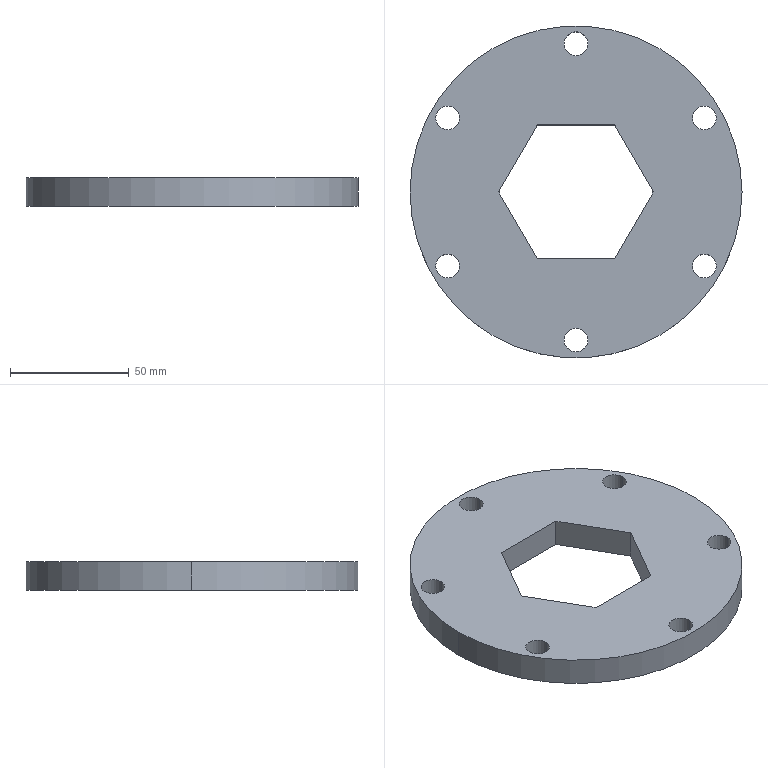Part | SolidWorks | features Extrusion 1 | 1 solid | 22 faces | box 140 x 140 x 12 mm | volume 145896 mm3 | cylinder 14 | plane 8 | commonest cylinder face diameters 10 x12 140 x2
STEP:
#1=CARTESIAN_POINT('',(-59.127,31.25,12.));
#2=VERTEX_POINT('',#1);
#3=CARTESIAN_POINT('',(-49.127,31.25,12.));
#4=VERTEX_POINT('',#3);
#5=CARTESIAN_POINT('',(-54.127,31.25,12.));
#6=DIRECTION('',(0.,0.,1.));
#7=DIRECTION('',(1.,0.,0.));
#8=AXIS2_PLACEMENT_3D('',#5,#6,#7);
#9=CIRCLE('',#8,5.);
#10=EDGE_CURVE('',#2,#4,#9,.T.);
#11=ORIENTED_EDGE('',*,*,#10,.T.);
#12=CARTESIAN_POINT('',(-49.127,31.25,0.));
#13=VERTEX_POINT('',#12);
#14=CARTESIAN_POINT('',(-49.127,31.25,12.));
#15=DIRECTION('',(0.,0.,-1.));
#16=VECTOR('',#15,1000.);
#17=LINE('',#14,#16);
#18=EDGE_CURVE('',#4,#13,#17,.T.);
#19=ORIENTED_EDGE('',*,*,#18,.T.);
#20=CARTESIAN_POINT('',(-59.127,31.25,0.));
#21=VERTEX_POINT('',#20);
#22=CARTESIAN_POINT('',(-54.127,31.25,0.));
#23=DIRECTION('',(0.,0.,1.));
#24=DIRECTION('',(1.,0.,0.));
#25=AXIS2_PLACEMENT_3D('',#22,#23,#24);
#26=CIRCLE('',#25,5.);
#27=EDGE_CURVE('',#21,#13,#26,.T.);
#28=ORIENTED_EDGE('',*,*,#27,.F.);
#29=CARTESIAN_POINT('',(-59.127,31.25,12.));
#30=DIRECTION('',(0.,0.,-1.));
#31=VECTOR('',#30,1000.);
#32=LINE('',#29,#31);
#33=EDGE_CURVE('',#2,#21,#32,.T.);
#34=ORIENTED_EDGE('',*,*,#33,.F.);
#35=EDGE_LOOP('',(#11,#19,#28,#34));
#36=FACE_OUTER_BOUND('',#35,.T.);
#37=CARTESIAN_POINT('',(-54.127,31.25,12.));
#38=DIRECTION('',(0.,0.,-1.));
#39=DIRECTION('',(-1.,0.,0.));
#40=AXIS2_PLACEMENT_3D('',#37,#38,#39);
#41=CYLINDRICAL_SURFACE('',#40,5.);
#42=ADVANCED_FACE('',(#36),#41,.F.);
#43=CARTESIAN_POINT('',(-59.127,-31.25,12.));
#44=VERTEX_POINT('',#43);
#45=CARTESIAN_POINT('',(-49.127,-31.25,12.));
#46=VERTEX_POINT('',#45);
#47=CARTESIAN_POINT('',(-54.127,-31.25,12.));
#48=DIRECTION('',(0.,0.,1.));
#49=DIRECTION('',(1.,0.,0.));
#50=AXIS2_PLACEMENT_3D('',#47,#48,#49);
#51=CIRCLE('',#50,5.);
#52=EDGE_CURVE('',#44,#46,#51,.T.);
#53=ORIENTED_EDGE('',*,*,#52,.T.);
#54=CARTESIAN_POINT('',(-49.127,-31.25,0.));
#55=VERTEX_POINT('',#54);
#56=CARTESIAN_POINT('',(-49.127,-31.25,12.));
#57=DIRECTION('',(0.,0.,-1.));
#58=VECTOR('',#57,1000.);
#59=LINE('',#56,#58);
#60=EDGE_CURVE('',#46,#55,#59,.T.);
#61=ORIENTED_EDGE('',*,*,#60,.T.);
#62=CARTESIAN_POINT('',(-59.127,-31.25,0.));
#63=VERTEX_POINT('',#62);
#64=CARTESIAN_POINT('',(-54.127,-31.25,0.));
#65=DIRECTION('',(0.,0.,1.));
#66=DIRECTION('',(1.,0.,0.));
#67=AXIS2_PLACEMENT_3D('',#64,#65,#66);
#68=CIRCLE('',#67,5.);
#69=EDGE_CURVE('',#63,#55,#68,.T.);
#70=ORIENTED_EDGE('',*,*,#69,.F.);
#71=CARTESIAN_POINT('',(-59.127,-31.25,12.));
#72=DIRECTION('',(0.,0.,-1.));
#73=VECTOR('',#72,1000.);
#74=LINE('',#71,#73);
#75=EDGE_CURVE('',#44,#63,#74,.T.);
#76=ORIENTED_EDGE('',*,*,#75,.F.);
#77=EDGE_LOOP('',(#53,#61,#70,#76));
#78=FACE_OUTER_BOUND('',#77,.T.);
#79=CARTESIAN_POINT('',(-54.127,-31.25,12.));
#80=DIRECTION('',(0.,0.,-1.));
#81=DIRECTION('',(-1.,0.,0.));
#82=AXIS2_PLACEMENT_3D('',#79,#80,#81);
#83=CYLINDRICAL_SURFACE('',#82,5.);
#84=ADVANCED_FACE('',(#78),#83,.F.);
#85=CARTESIAN_POINT('',(-5.,-62.5,12.));
#86=VERTEX_POINT('',#85);
#87=CARTESIAN_POINT('',(5.,-62.5,12.));
#88=VERTEX_POINT('',#87);
#89=CARTESIAN_POINT('',(0.,-62.5,12.));
#90=DIRECTION('',(0.,0.,1.));
#91=DIRECTION('',(1.,0.,0.));
#92=AXIS2_PLACEMENT_3D('',#89,#90,#91);
#93=CIRCLE('',#92,5.);
#94=EDGE_CURVE('',#86,#88,#93,.T.);
#95=ORIENTED_EDGE('',*,*,#94,.T.);
#96=CARTESIAN_POINT('',(5.,-62.5,0.));
#97=VERTEX_POINT('',#96);
#98=CARTESIAN_POINT('',(5.,-62.5,12.));
#99=DIRECTION('',(0.,0.,-1.));
#100=VECTOR('',#99,1000.);
#101=LINE('',#98,#100);
#102=EDGE_CURVE('',#88,#97,#101,.T.);
#103=ORIENTED_EDGE('',*,*,#102,.T.);
#104=CARTESIAN_POINT('',(-5.,-62.5,0.));
#105=VERTEX_POINT('',#104);
#106=CARTESIAN_POINT('',(0.,-62.5,0.));
#107=DIRECTION('',(0.,0.,1.));
#108=DIRECTION('',(1.,0.,0.));
#109=AXIS2_PLACEMENT_3D('',#106,#107,#108);
#110=CIRCLE('',#109,5.);
#111=EDGE_CURVE('',#105,#97,#110,.T.);
#112=ORIENTED_EDGE('',*,*,#111,.F.);
#113=CARTESIAN_POINT('',(-5.,-62.5,12.));
#114=DIRECTION('',(0.,0.,-1.));
#115=VECTOR('',#114,1000.);
#116=LINE('',#113,#115);
#117=EDGE_CURVE('',#86,#105,#116,.T.);
#118=ORIENTED_EDGE('',*,*,#117,.F.);
#119=EDGE_LOOP('',(#95,#103,#112,#118));
#120=FACE_OUTER_BOUND('',#119,.T.);
#121=CARTESIAN_POINT('',(0.,-62.5,12.));
#122=DIRECTION('',(0.,0.,-1.));
#123=DIRECTION('',(-1.,0.,0.));
#124=AXIS2_PLACEMENT_3D('',#121,#122,#123);
#125=CYLINDRICAL_SURFACE('',#124,5.);
#126=ADVANCED_FACE('',(#120),#125,.F.);
#127=CARTESIAN_POINT('',(49.127,-31.25,12.));
#128=VERTEX_POINT('',#127);
#129=CARTESIAN_POINT('',(59.127,-31.25,12.));
#130=VERTEX_POINT('',#129);
#131=CARTESIAN_POINT('',(54.127,-31.25,12.));
#132=DIRECTION('',(0.,0.,1.));
#133=DIRECTION('',(1.,0.,0.));
#134=AXIS2_PLACEMENT_3D('',#131,#132,#133);
#135=CIRCLE('',#134,5.);
#136=EDGE_CURVE('',#128,#130,#135,.T.);
#137=ORIENTED_EDGE('',*,*,#136,.T.);
#138=CARTESIAN_POINT('',(59.127,-31.25,0.));
#139=VERTEX_POINT('',#138);
#140=CARTESIAN_POINT('',(59.127,-31.25,12.));
#141=DIRECTION('',(0.,0.,-1.));
#142=VECTOR('',#141,1000.);
#143=LINE('',#140,#142);
#144=EDGE_CURVE('',#130,#139,#143,.T.);
#145=ORIENTED_EDGE('',*,*,#144,.T.);
#146=CARTESIAN_POINT('',(49.127,-31.25,0.));
#147=VERTEX_POINT('',#146);
#148=CARTESIAN_POINT('',(54.127,-31.25,0.));
#149=DIRECTION('',(0.,0.,1.));
#150=DIRECTION('',(1.,0.,0.));
#151=AXIS2_PLACEMENT_3D('',#148,#149,#150);
#152=CIRCLE('',#151,5.);
#153=EDGE_CURVE('',#147,#139,#152,.T.);
#154=ORIENTED_EDGE('',*,*,#153,.F.);
#155=CARTESIAN_POINT('',(49.127,-31.25,12.));
#156=DIRECTION('',(0.,0.,-1.));
#157=VECTOR('',#156,1000.);
#158=LINE('',#155,#157);
#159=EDGE_CURVE('',#128,#147,#158,.T.);
#160=ORIENTED_EDGE('',*,*,#159,.F.);
#161=EDGE_LOOP('',(#137,#145,#154,#160));
#162=FACE_OUTER_BOUND('',#161,.T.);
#163=CARTESIAN_POINT('',(54.127,-31.25,12.));
#164=DIRECTION('',(0.,0.,-1.));
#165=DIRECTION('',(-1.,0.,0.));
#166=AXIS2_PLACEMENT_3D('',#163,#164,#165);
#167=CYLINDRICAL_SURFACE('',#166,5.);
#168=ADVANCED_FACE('',(#162),#167,.F.);
#169=CARTESIAN_POINT('',(49.127,31.25,12.));
#170=VERTEX_POINT('',#169);
#171=CARTESIAN_POINT('',(59.127,31.25,12.));
#172=VERTEX_POINT('',#171);
#173=CARTESIAN_POINT('',(54.127,31.25,12.));
#174=DIRECTION('',(0.,0.,1.));
#175=DIRECTION('',(1.,0.,0.));
#176=AXIS2_PLACEMENT_3D('',#173,#174,#175);
#177=CIRCLE('',#176,5.);
#178=EDGE_CURVE('',#170,#172,#177,.T.);
#179=ORIENTED_EDGE('',*,*,#178,.T.);
#180=CARTESIAN_POINT('',(59.127,31.25,0.));
#181=VERTEX_POINT('',#180);
#182=CARTESIAN_POINT('',(59.127,31.25,12.));
#183=DIRECTION('',(0.,0.,-1.));
#184=VECTOR('',#183,1000.);
#185=LINE('',#182,#184);
#186=EDGE_CURVE('',#172,#181,#185,.T.);
#187=ORIENTED_EDGE('',*,*,#186,.T.);
#188=CARTESIAN_POINT('',(49.127,31.25,0.));
#189=VERTEX_POINT('',#188);
#190=CARTESIAN_POINT('',(54.127,31.25,0.));
#191=DIRECTION('',(0.,0.,1.));
#192=DIRECTION('',(1.,0.,0.));
#193=AXIS2_PLACEMENT_3D('',#190,#191,#192);
#194=CIRCLE('',#193,5.);
#195=EDGE_CURVE('',#189,#181,#194,.T.);
#196=ORIENTED_EDGE('',*,*,#195,.F.);
#197=CARTESIAN_POINT('',(49.127,31.25,12.));
#198=DIRECTION('',(0.,0.,-1.));
#199=VECTOR('',#198,1000.);
#200=LINE('',#197,#199);
#201=EDGE_CURVE('',#170,#189,#200,.T.);
#202=ORIENTED_EDGE('',*,*,#201,.F.);
#203=EDGE_LOOP('',(#179,#187,#196,#202));
#204=FACE_OUTER_BOUND('',#203,.T.);
#205=CARTESIAN_POINT('',(54.127,31.25,12.));
#206=DIRECTION('',(0.,0.,-1.));
#207=DIRECTION('',(-1.,0.,0.));
#208=AXIS2_PLACEMENT_3D('',#205,#206,#207);
#209=CYLINDRICAL_SURFACE('',#208,5.);
#210=ADVANCED_FACE('',(#204),#209,.F.);
#211=CARTESIAN_POINT('',(-5.,62.5,12.));
#212=VERTEX_POINT('',#211);
#213=CARTESIAN_POINT('',(5.,62.5,12.));
#214=VERTEX_POINT('',#213);
#215=CARTESIAN_POINT('',(0.,62.5,12.));
#216=DIRECTION('',(0.,0.,1.));
#217=DIRECTION('',(1.,0.,0.));
#218=AXIS2_PLACEMENT_3D('',#215,#216,#217);
#219=CIRCLE('',#218,5.);
#220=EDGE_CURVE('',#212,#214,#219,.T.);
#221=ORIENTED_EDGE('',*,*,#220,.T.);
#222=CARTESIAN_POINT('',(5.,62.5,0.));
#223=VERTEX_POINT('',#222);
#224=CARTESIAN_POINT('',(5.,62.5,12.));
#225=DIRECTION('',(0.,0.,-1.));
#226=VECTOR('',#225,1000.);
#227=LINE('',#224,#226);
#228=EDGE_CURVE('',#214,#223,#227,.T.);
#229=ORIENTED_EDGE('',*,*,#228,.T.);
#230=CARTESIAN_POINT('',(-5.,62.5,0.));
#231=VERTEX_POINT('',#230);
#232=CARTESIAN_POINT('',(0.,62.5,0.));
#233=DIRECTION('',(0.,0.,1.));
#234=DIRECTION('',(1.,0.,0.));
#235=AXIS2_PLACEMENT_3D('',#232,#233,#234);
#236=CIRCLE('',#235,5.);
#237=EDGE_CURVE('',#231,#223,#236,.T.);
#238=ORIENTED_EDGE('',*,*,#237,.F.);
#239=CARTESIAN_POINT('',(-5.,62.5,12.));
#240=DIRECTION('',(0.,0.,-1.));
#241=VECTOR('',#240,1000.);
#242=LINE('',#239,#241);
#243=EDGE_CURVE('',#212,#231,#242,.T.);
#244=ORIENTED_EDGE('',*,*,#243,.F.);
#245=EDGE_LOOP('',(#221,#229,#238,#244));
#246=FACE_OUTER_BOUND('',#245,.T.);
#247=CARTESIAN_POINT('',(0.,62.5,12.));
#248=DIRECTION('',(0.,0.,-1.));
#249=DIRECTION('',(-1.,0.,0.));
#250=AXIS2_PLACEMENT_3D('',#247,#248,#249);
#251=CYLINDRICAL_SURFACE('',#250,5.);
#252=ADVANCED_FACE('',(#246),#251,.F.);
#253=CARTESIAN_POINT('',(70.,0.,12.));
#254=VERTEX_POINT('',#253);
#255=CARTESIAN_POINT('',(-70.,0.,12.));
#256=VERTEX_POINT('',#255);
#257=CARTESIAN_POINT('',(0.,0.,12.));
#258=DIRECTION('',(0.,0.,1.));
#259=DIRECTION('',(1.,0.,0.));
#260=AXIS2_PLACEMENT_3D('',#257,#258,#259);
#261=CIRCLE('',#260,70.);
#262=EDGE_CURVE('',#254,#256,#261,.T.);
#263=ORIENTED_EDGE('',*,*,#262,.F.);
#264=CARTESIAN_POINT('',(70.,0.,0.));
#265=VERTEX_POINT('',#264);
#266=CARTESIAN_POINT('',(70.,0.,12.));
#267=DIRECTION('',(0.,0.,-1.));
#268=VECTOR('',#267,1000.);
#269=LINE('',#266,#268);
#270=EDGE_CURVE('',#254,#265,#269,.T.);
#271=ORIENTED_EDGE('',*,*,#270,.T.);
#272=CARTESIAN_POINT('',(-70.,0.,0.));
#273=VERTEX_POINT('',#272);
#274=CARTESIAN_POINT('',(0.,0.,0.));
#275=DIRECTION('',(0.,0.,1.));
#276=DIRECTION('',(1.,0.,0.));
#277=AXIS2_PLACEMENT_3D('',#274,#275,#276);
#278=CIRCLE('',#277,70.);
#279=EDGE_CURVE('',#265,#273,#278,.T.);
#280=ORIENTED_EDGE('',*,*,#279,.T.);
#281=CARTESIAN_POINT('',(-70.,0.,12.));
#282=DIRECTION('',(0.,0.,-1.));
#283=VECTOR('',#282,1000.);
#284=LINE('',#281,#283);
#285=EDGE_CURVE('',#256,#273,#284,.T.);
#286=ORIENTED_EDGE('',*,*,#285,.F.);
#287=EDGE_LOOP('',(#263,#271,#280,#286));
#288=FACE_OUTER_BOUND('',#287,.T.);
#289=CARTESIAN_POINT('',(0.,0.,12.));
#290=DIRECTION('',(0.,0.,-1.));
#291=DIRECTION('',(-1.,0.,0.));
#292=AXIS2_PLACEMENT_3D('',#289,#290,#291);
#293=CYLINDRICAL_SURFACE('',#292,70.);
#294=ADVANCED_FACE('',(#288),#293,.T.);
#295=ORIENTED_EDGE('',*,*,#52,.F.);
#296=CARTESIAN_POINT('',(-54.127,-31.25,12.));
#297=DIRECTION('',(0.,0.,1.));
#298=DIRECTION('',(1.,0.,0.));
#299=AXIS2_PLACEMENT_3D('',#296,#297,#298);
#300=CIRCLE('',#299,5.);
#301=EDGE_CURVE('',#46,#44,#300,.T.);
#302=ORIENTED_EDGE('',*,*,#301,.F.);
#303=EDGE_LOOP('',(#295,#302));
#304=FACE_BOUND('',#303,.T.);
#305=ORIENTED_EDGE('',*,*,#136,.F.);
#306=CARTESIAN_POINT('',(54.127,-31.25,12.));
#307=DIRECTION('',(0.,0.,1.));
#308=DIRECTION('',(1.,0.,0.));
#309=AXIS2_PLACEMENT_3D('',#306,#307,#308);
#310=CIRCLE('',#309,5.);
#311=EDGE_CURVE('',#130,#128,#310,.T.);
#312=ORIENTED_EDGE('',*,*,#311,.F.);
#313=EDGE_LOOP('',(#305,#312));
#314=FACE_BOUND('',#313,.T.);
#315=CARTESIAN_POINT('',(32.62,0.,12.));
#316=VERTEX_POINT('',#315);
#317=CARTESIAN_POINT('',(16.31,28.25,12.));
#318=VERTEX_POINT('',#317);
#319=CARTESIAN_POINT('',(32.62,0.,12.));
#320=DIRECTION('',(-0.5,0.866,0.));
#321=VECTOR('',#320,1000.);
#322=LINE('',#319,#321);
#323=EDGE_CURVE('',#316,#318,#322,.T.);
#324=ORIENTED_EDGE('',*,*,#323,.F.);
#325=CARTESIAN_POINT('',(16.31,-28.25,12.));
#326=VERTEX_POINT('',#325);
#327=CARTESIAN_POINT('',(16.31,-28.25,12.));
#328=DIRECTION('',(0.5,0.866,0.));
#329=VECTOR('',#328,1000.);
#330=LINE('',#327,#329);
#331=EDGE_CURVE('',#326,#316,#330,.T.);
#332=ORIENTED_EDGE('',*,*,#331,.F.);
#333=CARTESIAN_POINT('',(-16.31,-28.25,12.));
#334=VERTEX_POINT('',#333);
#335=CARTESIAN_POINT('',(-16.31,-28.25,12.));
#336=DIRECTION('',(1.,0.,0.));
#337=VECTOR('',#336,1000.);
#338=LINE('',#335,#337);
#339=EDGE_CURVE('',#334,#326,#338,.T.);
#340=ORIENTED_EDGE('',*,*,#339,.F.);
#341=CARTESIAN_POINT('',(-32.62,0.,12.));
#342=VERTEX_POINT('',#341);
#343=CARTESIAN_POINT('',(-32.62,0.,12.));
#344=DIRECTION('',(0.5,-0.866,0.));
#345=VECTOR('',#344,1000.);
#346=LINE('',#343,#345);
#347=EDGE_CURVE('',#342,#334,#346,.T.);
#348=ORIENTED_EDGE('',*,*,#347,.F.);
#349=CARTESIAN_POINT('',(-16.31,28.25,12.));
#350=VERTEX_POINT('',#349);
#351=CARTESIAN_POINT('',(-16.31,28.25,12.));
#352=DIRECTION('',(-0.5,-0.866,0.));
#353=VECTOR('',#352,1000.);
#354=LINE('',#351,#353);
#355=EDGE_CURVE('',#350,#342,#354,.T.);
#356=ORIENTED_EDGE('',*,*,#355,.F.);
#357=CARTESIAN_POINT('',(16.31,28.25,12.));
#358=DIRECTION('',(-1.,0.,0.));
#359=VECTOR('',#358,1000.);
#360=LINE('',#357,#359);
#361=EDGE_CURVE('',#318,#350,#360,.T.);
#362=ORIENTED_EDGE('',*,*,#361,.F.);
#363=EDGE_LOOP('',(#324,#332,#340,#348,#356,#362));
#364=FACE_BOUND('',#363,.T.);
#365=ORIENTED_EDGE('',*,*,#220,.F.);
#366=CARTESIAN_POINT('',(0.,62.5,12.));
#367=DIRECTION('',(0.,0.,1.));
#368=DIRECTION('',(1.,0.,0.));
#369=AXIS2_PLACEMENT_3D('',#366,#367,#368);
#370=CIRCLE('',#369,5.);
#371=EDGE_CURVE('',#214,#212,#370,.T.);
#372=ORIENTED_EDGE('',*,*,#371,.F.);
#373=EDGE_LOOP('',(#365,#372));
#374=FACE_BOUND('',#373,.T.);
#375=CARTESIAN_POINT('',(0.,0.,12.));
#376=DIRECTION('',(0.,0.,1.));
#377=DIRECTION('',(1.,0.,0.));
#378=AXIS2_PLACEMENT_3D('',#375,#376,#377);
#379=CIRCLE('',#378,70.);
#380=EDGE_CURVE('',#256,#254,#379,.T.);
#381=ORIENTED_EDGE('',*,*,#380,.T.);
#382=ORIENTED_EDGE('',*,*,#262,.T.);
#383=EDGE_LOOP('',(#381,#382));
#384=FACE_OUTER_BOUND('',#383,.T.);
#385=ORIENTED_EDGE('',*,*,#178,.F.);
#386=CARTESIAN_POINT('',(54.127,31.25,12.));
#387=DIRECTION('',(0.,0.,1.));
#388=DIRECTION('',(1.,0.,0.));
#389=AXIS2_PLACEMENT_3D('',#386,#387,#388);
#390=CIRCLE('',#389,5.);
#391=EDGE_CURVE('',#172,#170,#390,.T.);
#392=ORIENTED_EDGE('',*,*,#391,.F.);
#393=EDGE_LOOP('',(#385,#392));
#394=FACE_BOUND('',#393,.T.);
#395=ORIENTED_EDGE('',*,*,#94,.F.);
#396=CARTESIAN_POINT('',(0.,-62.5,12.));
#397=DIRECTION('',(0.,0.,1.));
#398=DIRECTION('',(1.,0.,0.));
#399=AXIS2_PLACEMENT_3D('',#396,#397,#398);
#400=CIRCLE('',#399,5.);
#401=EDGE_CURVE('',#88,#86,#400,.T.);
#402=ORIENTED_EDGE('',*,*,#401,.F.);
#403=EDGE_LOOP('',(#395,#402));
#404=FACE_BOUND('',#403,.T.);
#405=ORIENTED_EDGE('',*,*,#10,.F.);
#406=CARTESIAN_POINT('',(-54.127,31.25,12.));
#407=DIRECTION('',(0.,0.,1.));
#408=DIRECTION('',(1.,0.,0.));
#409=AXIS2_PLACEMENT_3D('',#406,#407,#408);
#410=CIRCLE('',#409,5.);
#411=EDGE_CURVE('',#4,#2,#410,.T.);
#412=ORIENTED_EDGE('',*,*,#411,.F.);
#413=EDGE_LOOP('',(#405,#412));
#414=FACE_BOUND('',#413,.T.);
#415=CARTESIAN_POINT('',(0.,0.,12.));
#416=DIRECTION('',(0.,0.,1.));
#417=DIRECTION('',(1.,0.,0.));
#418=AXIS2_PLACEMENT_3D('',#415,#416,#417);
#419=PLANE('',#418);
#420=ADVANCED_FACE('',(#304,#314,#364,#374,#384,#394,#404,#414),#419,.T.);
#421=ORIENTED_EDGE('',*,*,#237,.T.);
#422=CARTESIAN_POINT('',(0.,62.5,0.));
#423=DIRECTION('',(0.,0.,1.));
#424=DIRECTION('',(1.,0.,0.));
#425=AXIS2_PLACEMENT_3D('',#422,#423,#424);
#426=CIRCLE('',#425,5.);
#427=EDGE_CURVE('',#223,#231,#426,.T.);
#428=ORIENTED_EDGE('',*,*,#427,.T.);
#429=EDGE_LOOP('',(#421,#428));
#430=FACE_BOUND('',#429,.T.);
#431=CARTESIAN_POINT('',(0.,0.,0.));
#432=DIRECTION('',(0.,0.,1.));
#433=DIRECTION('',(1.,0.,0.));
#434=AXIS2_PLACEMENT_3D('',#431,#432,#433);
#435=CIRCLE('',#434,70.);
#436=EDGE_CURVE('',#273,#265,#435,.T.);
#437=ORIENTED_EDGE('',*,*,#436,.F.);
#438=ORIENTED_EDGE('',*,*,#279,.F.);
#439=EDGE_LOOP('',(#437,#438));
#440=FACE_OUTER_BOUND('',#439,.T.);
#441=CARTESIAN_POINT('',(16.31,-28.25,0.));
#442=VERTEX_POINT('',#441);
#443=CARTESIAN_POINT('',(32.62,0.,0.));
#444=VERTEX_POINT('',#443);
#445=CARTESIAN_POINT('',(16.31,-28.25,0.));
#446=DIRECTION('',(0.5,0.866,0.));
#447=VECTOR('',#446,1000.);
#448=LINE('',#445,#447);
#449=EDGE_CURVE('',#442,#444,#448,.T.);
#450=ORIENTED_EDGE('',*,*,#449,.T.);
#451=CARTESIAN_POINT('',(16.31,28.25,0.));
#452=VERTEX_POINT('',#451);
#453=CARTESIAN_POINT('',(32.62,0.,0.));
#454=DIRECTION('',(-0.5,0.866,0.));
#455=VECTOR('',#454,1000.);
#456=LINE('',#453,#455);
#457=EDGE_CURVE('',#444,#452,#456,.T.);
#458=ORIENTED_EDGE('',*,*,#457,.T.);
#459=CARTESIAN_POINT('',(-16.31,28.25,0.));
#460=VERTEX_POINT('',#459);
#461=CARTESIAN_POINT('',(16.31,28.25,0.));
#462=DIRECTION('',(-1.,0.,0.));
#463=VECTOR('',#462,1000.);
#464=LINE('',#461,#463);
#465=EDGE_CURVE('',#452,#460,#464,.T.);
#466=ORIENTED_EDGE('',*,*,#465,.T.);
#467=CARTESIAN_POINT('',(-32.62,0.,0.));
#468=VERTEX_POINT('',#467);
#469=CARTESIAN_POINT('',(-16.31,28.25,0.));
#470=DIRECTION('',(-0.5,-0.866,0.));
#471=VECTOR('',#470,1000.);
#472=LINE('',#469,#471);
#473=EDGE_CURVE('',#460,#468,#472,.T.);
#474=ORIENTED_EDGE('',*,*,#473,.T.);
#475=CARTESIAN_POINT('',(-16.31,-28.25,0.));
#476=VERTEX_POINT('',#475);
#477=CARTESIAN_POINT('',(-32.62,0.,0.));
#478=DIRECTION('',(0.5,-0.866,0.));
#479=VECTOR('',#478,1000.);
#480=LINE('',#477,#479);
#481=EDGE_CURVE('',#468,#476,#480,.T.);
#482=ORIENTED_EDGE('',*,*,#481,.T.);
#483=CARTESIAN_POINT('',(-16.31,-28.25,0.));
#484=DIRECTION('',(1.,0.,0.));
#485=VECTOR('',#484,1000.);
#486=LINE('',#483,#485);
#487=EDGE_CURVE('',#476,#442,#486,.T.);
#488=ORIENTED_EDGE('',*,*,#487,.T.);
#489=EDGE_LOOP('',(#450,#458,#466,#474,#482,#488));
#490=FACE_BOUND('',#489,.T.);
#491=ORIENTED_EDGE('',*,*,#195,.T.);
#492=CARTESIAN_POINT('',(54.127,31.25,0.));
#493=DIRECTION('',(0.,0.,1.));
#494=DIRECTION('',(1.,0.,0.));
#495=AXIS2_PLACEMENT_3D('',#492,#493,#494);
#496=CIRCLE('',#495,5.);
#497=EDGE_CURVE('',#181,#189,#496,.T.);
#498=ORIENTED_EDGE('',*,*,#497,.T.);
#499=EDGE_LOOP('',(#491,#498));
#500=FACE_BOUND('',#499,.T.);
#501=ORIENTED_EDGE('',*,*,#153,.T.);
#502=CARTESIAN_POINT('',(54.127,-31.25,0.));
#503=DIRECTION('',(0.,0.,1.));
#504=DIRECTION('',(1.,0.,0.));
#505=AXIS2_PLACEMENT_3D('',#502,#503,#504);
#506=CIRCLE('',#505,5.);
#507=EDGE_CURVE('',#139,#147,#506,.T.);
#508=ORIENTED_EDGE('',*,*,#507,.T.);
#509=EDGE_LOOP('',(#501,#508));
#510=FACE_BOUND('',#509,.T.);
#511=ORIENTED_EDGE('',*,*,#111,.T.);
#512=CARTESIAN_POINT('',(0.,-62.5,0.));
#513=DIRECTION('',(0.,0.,1.));
#514=DIRECTION('',(1.,0.,0.));
#515=AXIS2_PLACEMENT_3D('',#512,#513,#514);
#516=CIRCLE('',#515,5.);
#517=EDGE_CURVE('',#97,#105,#516,.T.);
#518=ORIENTED_EDGE('',*,*,#517,.T.);
#519=EDGE_LOOP('',(#511,#518));
#520=FACE_BOUND('',#519,.T.);
#521=ORIENTED_EDGE('',*,*,#69,.T.);
#522=CARTESIAN_POINT('',(-54.127,-31.25,0.));
#523=DIRECTION('',(0.,0.,1.));
#524=DIRECTION('',(1.,0.,0.));
#525=AXIS2_PLACEMENT_3D('',#522,#523,#524);
#526=CIRCLE('',#525,5.);
#527=EDGE_CURVE('',#55,#63,#526,.T.);
#528=ORIENTED_EDGE('',*,*,#527,.T.);
#529=EDGE_LOOP('',(#521,#528));
#530=FACE_BOUND('',#529,.T.);
#531=ORIENTED_EDGE('',*,*,#27,.T.);
#532=CARTESIAN_POINT('',(-54.127,31.25,0.));
#533=DIRECTION('',(0.,0.,1.));
#534=DIRECTION('',(1.,0.,0.));
#535=AXIS2_PLACEMENT_3D('',#532,#533,#534);
#536=CIRCLE('',#535,5.);
#537=EDGE_CURVE('',#13,#21,#536,.T.);
#538=ORIENTED_EDGE('',*,*,#537,.T.);
#539=EDGE_LOOP('',(#531,#538));
#540=FACE_BOUND('',#539,.T.);
#541=CARTESIAN_POINT('',(0.,0.,0.));
#542=DIRECTION('',(0.,0.,1.));
#543=DIRECTION('',(1.,0.,0.));
#544=AXIS2_PLACEMENT_3D('',#541,#542,#543);
#545=PLANE('',#544);
#546=ADVANCED_FACE('',(#430,#440,#490,#500,#510,#520,#530,#540),#545,.F.);
#547=ORIENTED_EDGE('',*,*,#270,.F.);
#548=ORIENTED_EDGE('',*,*,#380,.F.);
#549=ORIENTED_EDGE('',*,*,#285,.T.);
#550=ORIENTED_EDGE('',*,*,#436,.T.);
#551=EDGE_LOOP('',(#547,#548,#549,#550));
#552=FACE_OUTER_BOUND('',#551,.T.);
#553=CARTESIAN_POINT('',(0.,0.,12.));
#554=DIRECTION('',(0.,0.,-1.));
#555=DIRECTION('',(-1.,0.,0.));
#556=AXIS2_PLACEMENT_3D('',#553,#554,#555);
#557=CYLINDRICAL_SURFACE('',#556,70.);
#558=ADVANCED_FACE('',(#552),#557,.T.);
#559=ORIENTED_EDGE('',*,*,#228,.F.);
#560=ORIENTED_EDGE('',*,*,#371,.T.);
#561=ORIENTED_EDGE('',*,*,#243,.T.);
#562=ORIENTED_EDGE('',*,*,#427,.F.);
#563=EDGE_LOOP('',(#559,#560,#561,#562));
#564=FACE_OUTER_BOUND('',#563,.T.);
#565=CARTESIAN_POINT('',(0.,62.5,12.));
#566=DIRECTION('',(0.,0.,-1.));
#567=DIRECTION('',(-1.,0.,0.));
#568=AXIS2_PLACEMENT_3D('',#565,#566,#567);
#569=CYLINDRICAL_SURFACE('',#568,5.);
#570=ADVANCED_FACE('',(#564),#569,.F.);
#571=ORIENTED_EDGE('',*,*,#449,.F.);
#572=CARTESIAN_POINT('',(16.31,-28.25,12.));
#573=DIRECTION('',(0.,0.,-1.));
#574=VECTOR('',#573,1000.);
#575=LINE('',#572,#574);
#576=EDGE_CURVE('',#326,#442,#575,.T.);
#577=ORIENTED_EDGE('',*,*,#576,.F.);
#578=ORIENTED_EDGE('',*,*,#331,.T.);
#579=CARTESIAN_POINT('',(32.62,0.,12.));
#580=DIRECTION('',(0.,0.,-1.));
#581=VECTOR('',#580,1000.);
#582=LINE('',#579,#581);
#583=EDGE_CURVE('',#316,#444,#582,.T.);
#584=ORIENTED_EDGE('',*,*,#583,.T.);
#585=EDGE_LOOP('',(#571,#577,#578,#584));
#586=FACE_OUTER_BOUND('',#585,.T.);
#587=CARTESIAN_POINT('',(16.31,-28.25,12.));
#588=DIRECTION('',(-0.866,0.5,0.));
#589=DIRECTION('',(-0.5,-0.866,0.));
#590=AXIS2_PLACEMENT_3D('',#587,#588,#589);
#591=PLANE('',#590);
#592=ADVANCED_FACE('',(#586),#591,.T.);
#593=ORIENTED_EDGE('',*,*,#457,.F.);
#594=ORIENTED_EDGE('',*,*,#583,.F.);
#595=ORIENTED_EDGE('',*,*,#323,.T.);
#596=CARTESIAN_POINT('',(16.31,28.25,12.));
#597=DIRECTION('',(0.,0.,-1.));
#598=VECTOR('',#597,1000.);
#599=LINE('',#596,#598);
#600=EDGE_CURVE('',#318,#452,#599,.T.);
#601=ORIENTED_EDGE('',*,*,#600,.T.);
#602=EDGE_LOOP('',(#593,#594,#595,#601));
#603=FACE_OUTER_BOUND('',#602,.T.);
#604=CARTESIAN_POINT('',(32.62,0.,12.));
#605=DIRECTION('',(-0.866,-0.5,0.));
#606=DIRECTION('',(0.5,-0.866,0.));
#607=AXIS2_PLACEMENT_3D('',#604,#605,#606);
#608=PLANE('',#607);
#609=ADVANCED_FACE('',(#603),#608,.T.);
#610=ORIENTED_EDGE('',*,*,#465,.F.);
#611=ORIENTED_EDGE('',*,*,#600,.F.);
#612=ORIENTED_EDGE('',*,*,#361,.T.);
#613=CARTESIAN_POINT('',(-16.31,28.25,12.));
#614=DIRECTION('',(0.,0.,-1.));
#615=VECTOR('',#614,1000.);
#616=LINE('',#613,#615);
#617=EDGE_CURVE('',#350,#460,#616,.T.);
#618=ORIENTED_EDGE('',*,*,#617,.T.);
#619=EDGE_LOOP('',(#610,#611,#612,#618));
#620=FACE_OUTER_BOUND('',#619,.T.);
#621=CARTESIAN_POINT('',(16.31,28.25,12.));
#622=DIRECTION('',(0.,-1.,0.));
#623=DIRECTION('',(0.,0.,-1.));
#624=AXIS2_PLACEMENT_3D('',#621,#622,#623);
#625=PLANE('',#624);
#626=ADVANCED_FACE('',(#620),#625,.T.);
#627=ORIENTED_EDGE('',*,*,#473,.F.);
#628=ORIENTED_EDGE('',*,*,#617,.F.);
#629=ORIENTED_EDGE('',*,*,#355,.T.);
#630=CARTESIAN_POINT('',(-32.62,0.,12.));
#631=DIRECTION('',(0.,0.,-1.));
#632=VECTOR('',#631,1000.);
#633=LINE('',#630,#632);
#634=EDGE_CURVE('',#342,#468,#633,.T.);
#635=ORIENTED_EDGE('',*,*,#634,.T.);
#636=EDGE_LOOP('',(#627,#628,#629,#635));
#637=FACE_OUTER_BOUND('',#636,.T.);
#638=CARTESIAN_POINT('',(-16.31,28.25,12.));
#639=DIRECTION('',(0.866,-0.5,0.));
#640=DIRECTION('',(0.5,0.866,0.));
#641=AXIS2_PLACEMENT_3D('',#638,#639,#640);
#642=PLANE('',#641);
#643=ADVANCED_FACE('',(#637),#642,.T.);
#644=ORIENTED_EDGE('',*,*,#481,.F.);
#645=ORIENTED_EDGE('',*,*,#634,.F.);
#646=ORIENTED_EDGE('',*,*,#347,.T.);
#647=CARTESIAN_POINT('',(-16.31,-28.25,12.));
#648=DIRECTION('',(0.,0.,-1.));
#649=VECTOR('',#648,1000.);
#650=LINE('',#647,#649);
#651=EDGE_CURVE('',#334,#476,#650,.T.);
#652=ORIENTED_EDGE('',*,*,#651,.T.);
#653=EDGE_LOOP('',(#644,#645,#646,#652));
#654=FACE_OUTER_BOUND('',#653,.T.);
#655=CARTESIAN_POINT('',(-32.62,0.,12.));
#656=DIRECTION('',(0.866,0.5,0.));
#657=DIRECTION('',(-0.5,0.866,0.));
#658=AXIS2_PLACEMENT_3D('',#655,#656,#657);
#659=PLANE('',#658);
#660=ADVANCED_FACE('',(#654),#659,.T.);
#661=ORIENTED_EDGE('',*,*,#487,.F.);
#662=ORIENTED_EDGE('',*,*,#651,.F.);
#663=ORIENTED_EDGE('',*,*,#339,.T.);
#664=ORIENTED_EDGE('',*,*,#576,.T.);
#665=EDGE_LOOP('',(#661,#662,#663,#664));
#666=FACE_OUTER_BOUND('',#665,.T.);
#667=CARTESIAN_POINT('',(-16.31,-28.25,12.));
#668=DIRECTION('',(0.,1.,0.));
#669=DIRECTION('',(-1.,0.,0.));
#670=AXIS2_PLACEMENT_3D('',#667,#668,#669);
#671=PLANE('',#670);
#672=ADVANCED_FACE('',(#666),#671,.T.);
#673=ORIENTED_EDGE('',*,*,#186,.F.);
#674=ORIENTED_EDGE('',*,*,#391,.T.);
#675=ORIENTED_EDGE('',*,*,#201,.T.);
#676=ORIENTED_EDGE('',*,*,#497,.F.);
#677=EDGE_LOOP('',(#673,#674,#675,#676));
#678=FACE_OUTER_BOUND('',#677,.T.);
#679=CARTESIAN_POINT('',(54.127,31.25,12.));
#680=DIRECTION('',(0.,0.,-1.));
#681=DIRECTION('',(-1.,0.,0.));
#682=AXIS2_PLACEMENT_3D('',#679,#680,#681);
#683=CYLINDRICAL_SURFACE('',#682,5.);
#684=ADVANCED_FACE('',(#678),#683,.F.);
#685=ORIENTED_EDGE('',*,*,#144,.F.);
#686=ORIENTED_EDGE('',*,*,#311,.T.);
#687=ORIENTED_EDGE('',*,*,#159,.T.);
#688=ORIENTED_EDGE('',*,*,#507,.F.);
#689=EDGE_LOOP('',(#685,#686,#687,#688));
#690=FACE_OUTER_BOUND('',#689,.T.);
#691=CARTESIAN_POINT('',(54.127,-31.25,12.));
#692=DIRECTION('',(0.,0.,-1.));
#693=DIRECTION('',(-1.,0.,0.));
#694=AXIS2_PLACEMENT_3D('',#691,#692,#693);
#695=CYLINDRICAL_SURFACE('',#694,5.);
#696=ADVANCED_FACE('',(#690),#695,.F.);
#697=ORIENTED_EDGE('',*,*,#102,.F.);
#698=ORIENTED_EDGE('',*,*,#401,.T.);
#699=ORIENTED_EDGE('',*,*,#117,.T.);
#700=ORIENTED_EDGE('',*,*,#517,.F.);
#701=EDGE_LOOP('',(#697,#698,#699,#700));
#702=FACE_OUTER_BOUND('',#701,.T.);
#703=CARTESIAN_POINT('',(0.,-62.5,12.));
#704=DIRECTION('',(0.,0.,-1.));
#705=DIRECTION('',(-1.,0.,0.));
#706=AXIS2_PLACEMENT_3D('',#703,#704,#705);
#707=CYLINDRICAL_SURFACE('',#706,5.);
#708=ADVANCED_FACE('',(#702),#707,.F.);
#709=ORIENTED_EDGE('',*,*,#60,.F.);
#710=ORIENTED_EDGE('',*,*,#301,.T.);
#711=ORIENTED_EDGE('',*,*,#75,.T.);
#712=ORIENTED_EDGE('',*,*,#527,.F.);
#713=EDGE_LOOP('',(#709,#710,#711,#712));
#714=FACE_OUTER_BOUND('',#713,.T.);
#715=CARTESIAN_POINT('',(-54.127,-31.25,12.));
#716=DIRECTION('',(0.,0.,-1.));
#717=DIRECTION('',(-1.,0.,0.));
#718=AXIS2_PLACEMENT_3D('',#715,#716,#717);
#719=CYLINDRICAL_SURFACE('',#718,5.);
#720=ADVANCED_FACE('',(#714),#719,.F.);
#721=ORIENTED_EDGE('',*,*,#18,.F.);
#722=ORIENTED_EDGE('',*,*,#411,.T.);
#723=ORIENTED_EDGE('',*,*,#33,.T.);
#724=ORIENTED_EDGE('',*,*,#537,.F.);
#725=EDGE_LOOP('',(#721,#722,#723,#724));
#726=FACE_OUTER_BOUND('',#725,.T.);
#727=CARTESIAN_POINT('',(-54.127,31.25,12.));
#728=DIRECTION('',(0.,0.,-1.));
#729=DIRECTION('',(-1.,0.,0.));
#730=AXIS2_PLACEMENT_3D('',#727,#728,#729);
#731=CYLINDRICAL_SURFACE('',#730,5.);
#732=ADVANCED_FACE('',(#726),#731,.F.);
#733=CLOSED_SHELL('',(#42,#84,#126,#168,#210,#252,#294,#420,#546,#558,#570,#592,#609,#626,#643,#660,#672,#684,#696,#708,#720,#732));
#734=MANIFOLD_SOLID_BREP('',#733);
#735=CARTESIAN_POINT('',(0.,0.,0.));
#736=DIRECTION('',(0.,0.,1.));
#737=DIRECTION('',(1.,0.,0.));
#738=AXIS2_PLACEMENT_3D('',#735,#736,#737);
#739=(LENGTH_UNIT()NAMED_UNIT(*)SI_UNIT(.MILLI.,.METRE.));
#740=UNCERTAINTY_MEASURE_WITH_UNIT(LENGTH_MEASURE(0.00001),#739,'','');
#741=(NAMED_UNIT(*)PLANE_ANGLE_UNIT()SI_UNIT($,.RADIAN.));
#742=(NAMED_UNIT(*)SI_UNIT($,.STERADIAN.)SOLID_ANGLE_UNIT());
#743=(GEOMETRIC_REPRESENTATION_CONTEXT(3)GLOBAL_UNCERTAINTY_ASSIGNED_CONTEXT((#740))GLOBAL_UNIT_ASSIGNED_CONTEXT((#739,#741,#742))REPRESENTATION_CONTEXT('',''));
#744=ADVANCED_BREP_SHAPE_REPRESENTATION('',(#734,#738),#743);